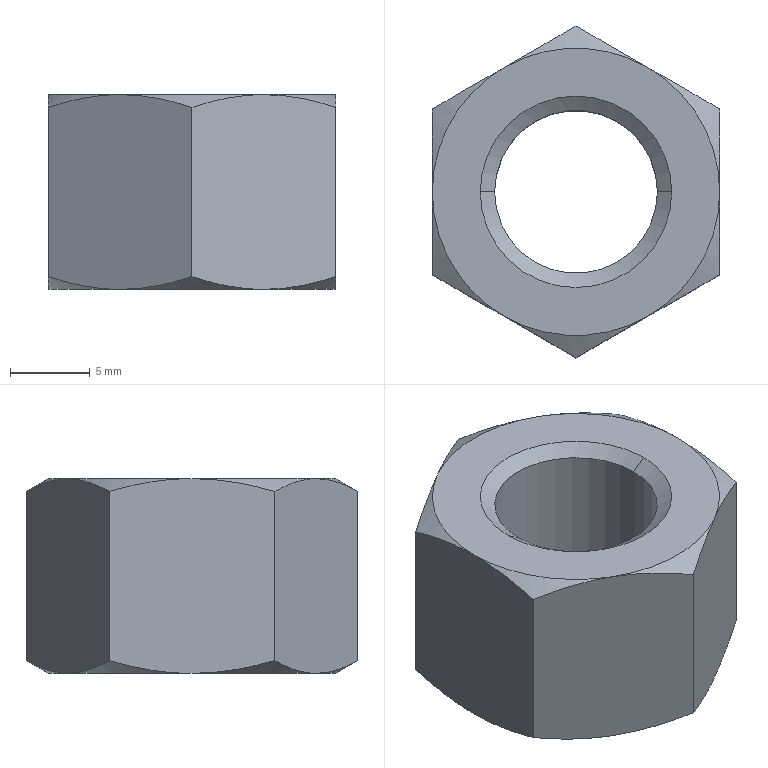Part | STEP file | hex nut gradec_iso_ISO - 4034 - M12 - N | 1 solid | 28 faces | box 18 x 20.785 x 12.2 mm | volume 2394 mm3 | cone 16 | plane 8 | cylinder 4 | commonest cylinder face diameters 10.2 x2 12 x2
STEP:
#1=CARTESIAN_POINT('',(-6.,0.,-12.2));
#2=VERTEX_POINT('',#1);
#3=CARTESIAN_POINT('',(6.,0.,-12.2));
#4=VERTEX_POINT('',#3);
#5=CARTESIAN_POINT('',(0.,0.,-12.2));
#6=DIRECTION('',(0.,0.,1.));
#7=DIRECTION('',(-1.,0.,0.));
#8=AXIS2_PLACEMENT_3D('',#5,#6,#7);
#9=CIRCLE('',#8,6.);
#10=EDGE_CURVE('',#2,#4,#9,.T.);
#11=ORIENTED_EDGE('',*,*,#10,.F.);
#12=CARTESIAN_POINT('',(-6.,0.,-12.175));
#13=VERTEX_POINT('',#12);
#14=CARTESIAN_POINT('',(-6.,0.,-25.038));
#15=DIRECTION('',(0.,0.,1.));
#16=VECTOR('',#15,1000.);
#17=LINE('',#14,#16);
#18=EDGE_CURVE('',#2,#13,#17,.T.);
#19=ORIENTED_EDGE('',*,*,#18,.T.);
#20=CARTESIAN_POINT('',(6.,0.,-12.175));
#21=VERTEX_POINT('',#20);
#22=CARTESIAN_POINT('',(0.,0.,-12.175));
#23=DIRECTION('',(0.,0.,1.));
#24=DIRECTION('',(1.,0.,0.));
#25=AXIS2_PLACEMENT_3D('',#22,#23,#24);
#26=CIRCLE('',#25,6.);
#27=EDGE_CURVE('',#13,#21,#26,.T.);
#28=ORIENTED_EDGE('',*,*,#27,.T.);
#29=CARTESIAN_POINT('',(6.,0.,-25.038));
#30=DIRECTION('',(0.,0.,1.));
#31=VECTOR('',#30,1000.);
#32=LINE('',#29,#31);
#33=EDGE_CURVE('',#4,#21,#32,.T.);
#34=ORIENTED_EDGE('',*,*,#33,.F.);
#35=EDGE_LOOP('',(#11,#19,#28,#34));
#36=FACE_OUTER_BOUND('',#35,.T.);
#37=CARTESIAN_POINT('',(0.,0.,-25.038));
#38=DIRECTION('',(0.,0.,1.));
#39=DIRECTION('',(1.,0.,0.));
#40=AXIS2_PLACEMENT_3D('',#37,#38,#39);
#41=CYLINDRICAL_SURFACE('',#40,6.);
#42=ADVANCED_FACE('',(#36),#41,.F.);
#43=CARTESIAN_POINT('',(-5.1,0.,-11.544));
#44=VERTEX_POINT('',#43);
#45=CARTESIAN_POINT('',(5.1,0.,-11.544));
#46=VERTEX_POINT('',#45);
#47=CARTESIAN_POINT('',(0.,0.,-11.544));
#48=DIRECTION('',(0.,0.,1.));
#49=DIRECTION('',(-1.,0.,0.));
#50=AXIS2_PLACEMENT_3D('',#47,#48,#49);
#51=CIRCLE('',#50,5.1);
#52=EDGE_CURVE('',#44,#46,#51,.T.);
#53=ORIENTED_EDGE('',*,*,#52,.T.);
#54=CARTESIAN_POINT('',(6.,0.,-12.175));
#55=DIRECTION('',(0.8192,0.,-0.5736));
#56=VECTOR('',#55,1000.);
#57=LINE('',#54,#56);
#58=EDGE_CURVE('',#46,#21,#57,.T.);
#59=ORIENTED_EDGE('',*,*,#58,.T.);
#60=ORIENTED_EDGE('',*,*,#27,.F.);
#61=CARTESIAN_POINT('',(-6.,0.,-12.175));
#62=DIRECTION('',(-0.8192,0.,-0.5736));
#63=VECTOR('',#62,1000.);
#64=LINE('',#61,#63);
#65=EDGE_CURVE('',#44,#13,#64,.T.);
#66=ORIENTED_EDGE('',*,*,#65,.F.);
#67=EDGE_LOOP('',(#53,#59,#60,#66));
#68=FACE_OUTER_BOUND('',#67,.T.);
#69=CARTESIAN_POINT('',(0.,0.,-12.175));
#70=DIRECTION('',(0.,0.,-1.));
#71=DIRECTION('',(-1.,0.,0.));
#72=AXIS2_PLACEMENT_3D('',#69,#70,#71);
#73=CONICAL_SURFACE('',#72,6.,0.9599);
#74=ADVANCED_FACE('',(#68),#73,.F.);
#75=CARTESIAN_POINT('',(5.1,0.,-0.6302));
#76=VERTEX_POINT('',#75);
#77=CARTESIAN_POINT('',(-5.1,0.,-0.6302));
#78=VERTEX_POINT('',#77);
#79=CARTESIAN_POINT('',(0.,0.,-0.6302));
#80=DIRECTION('',(0.,0.,-1.));
#81=DIRECTION('',(1.,0.,0.));
#82=AXIS2_PLACEMENT_3D('',#79,#80,#81);
#83=CIRCLE('',#82,5.1);
#84=EDGE_CURVE('',#76,#78,#83,.T.);
#85=ORIENTED_EDGE('',*,*,#84,.T.);
#86=CARTESIAN_POINT('',(-6.,0.,0.));
#87=VERTEX_POINT('',#86);
#88=CARTESIAN_POINT('',(-5.01,0.,-0.6932));
#89=DIRECTION('',(-0.8192,0.,0.5736));
#90=VECTOR('',#89,1000.);
#91=LINE('',#88,#90);
#92=EDGE_CURVE('',#78,#87,#91,.T.);
#93=ORIENTED_EDGE('',*,*,#92,.T.);
#94=CARTESIAN_POINT('',(6.,0.,0.));
#95=VERTEX_POINT('',#94);
#96=CARTESIAN_POINT('',(0.,0.,0.));
#97=DIRECTION('',(0.,0.,1.));
#98=DIRECTION('',(1.,0.,0.));
#99=AXIS2_PLACEMENT_3D('',#96,#97,#98);
#100=CIRCLE('',#99,6.);
#101=EDGE_CURVE('',#87,#95,#100,.T.);
#102=ORIENTED_EDGE('',*,*,#101,.T.);
#103=CARTESIAN_POINT('',(5.01,0.,-0.6932));
#104=DIRECTION('',(0.8192,0.,0.5736));
#105=VECTOR('',#104,1000.);
#106=LINE('',#103,#105);
#107=EDGE_CURVE('',#76,#95,#106,.T.);
#108=ORIENTED_EDGE('',*,*,#107,.F.);
#109=EDGE_LOOP('',(#85,#93,#102,#108));
#110=FACE_OUTER_BOUND('',#109,.T.);
#111=CARTESIAN_POINT('',(0.,0.,-0.6932));
#112=DIRECTION('',(0.,0.,1.));
#113=DIRECTION('',(1.,0.,0.));
#114=AXIS2_PLACEMENT_3D('',#111,#112,#113);
#115=CONICAL_SURFACE('',#114,5.01,0.9599);
#116=ADVANCED_FACE('',(#110),#115,.F.);
#117=ORIENTED_EDGE('',*,*,#52,.F.);
#118=CARTESIAN_POINT('',(-5.1,0.,-12.2));
#119=DIRECTION('',(0.,0.,1.));
#120=VECTOR('',#119,1000.);
#121=LINE('',#118,#120);
#122=EDGE_CURVE('',#44,#78,#121,.T.);
#123=ORIENTED_EDGE('',*,*,#122,.T.);
#124=ORIENTED_EDGE('',*,*,#84,.F.);
#125=CARTESIAN_POINT('',(5.1,0.,-12.2));
#126=DIRECTION('',(0.,0.,1.));
#127=VECTOR('',#126,1000.);
#128=LINE('',#125,#127);
#129=EDGE_CURVE('',#46,#76,#128,.T.);
#130=ORIENTED_EDGE('',*,*,#129,.F.);
#131=EDGE_LOOP('',(#117,#123,#124,#130));
#132=FACE_OUTER_BOUND('',#131,.T.);
#133=CARTESIAN_POINT('',(0.,0.,-12.2));
#134=DIRECTION('',(0.,0.,1.));
#135=DIRECTION('',(1.,0.,0.));
#136=AXIS2_PLACEMENT_3D('',#133,#134,#135);
#137=CYLINDRICAL_SURFACE('',#136,5.1);
#138=ADVANCED_FACE('',(#132),#137,.F.);
#139=ORIENTED_EDGE('',*,*,#122,.F.);
#140=CARTESIAN_POINT('',(0.,0.,-11.544));
#141=DIRECTION('',(0.,0.,1.));
#142=DIRECTION('',(-1.,0.,0.));
#143=AXIS2_PLACEMENT_3D('',#140,#141,#142);
#144=CIRCLE('',#143,5.1);
#145=EDGE_CURVE('',#46,#44,#144,.T.);
#146=ORIENTED_EDGE('',*,*,#145,.F.);
#147=ORIENTED_EDGE('',*,*,#129,.T.);
#148=CARTESIAN_POINT('',(0.,0.,-0.6302));
#149=DIRECTION('',(0.,0.,-1.));
#150=DIRECTION('',(1.,0.,0.));
#151=AXIS2_PLACEMENT_3D('',#148,#149,#150);
#152=CIRCLE('',#151,5.1);
#153=EDGE_CURVE('',#78,#76,#152,.T.);
#154=ORIENTED_EDGE('',*,*,#153,.F.);
#155=EDGE_LOOP('',(#139,#146,#147,#154));
#156=FACE_OUTER_BOUND('',#155,.T.);
#157=CARTESIAN_POINT('',(0.,0.,-12.2));
#158=DIRECTION('',(0.,0.,1.));
#159=DIRECTION('',(1.,0.,0.));
#160=AXIS2_PLACEMENT_3D('',#157,#158,#159);
#161=CYLINDRICAL_SURFACE('',#160,5.1);
#162=ADVANCED_FACE('',(#156),#161,.F.);
#163=CARTESIAN_POINT('',(-9.,5.196,-11.396));
#164=VERTEX_POINT('',#163);
#165=CARTESIAN_POINT('',(-9.,5.196,-0.8038));
#166=VERTEX_POINT('',#165);
#167=CARTESIAN_POINT('',(-9.,5.196,-12.2));
#168=DIRECTION('',(0.,0.,1.));
#169=VECTOR('',#168,1000.);
#170=LINE('',#167,#169);
#171=EDGE_CURVE('',#164,#166,#170,.T.);
#172=ORIENTED_EDGE('',*,*,#171,.T.);
#173=CARTESIAN_POINT('',(-4.5,7.794,0.));
#174=VERTEX_POINT('',#173);
#175=CARTESIAN_POINT('',(-9.,5.196,-0.8038));
#176=CARTESIAN_POINT('',(-8.264,5.621,-0.5585));
#177=CARTESIAN_POINT('',(-7.522,6.049,-0.3563));
#178=CARTESIAN_POINT('',(-6.024,6.914,-0.07661));
#179=CARTESIAN_POINT('',(-5.267,7.352,0.));
#180=CARTESIAN_POINT('',(-4.5,7.794,0.));
#181=B_SPLINE_CURVE_WITH_KNOTS('',3,(#175,#176,#177,#178,#179,#180),.UNSPECIFIED.,.F.,.F.,(4,2,4),(0.000000238,0.002629,0.005258),.UNSPECIFIED.);
#182=EDGE_CURVE('',#166,#174,#181,.T.);
#183=ORIENTED_EDGE('',*,*,#182,.T.);
#184=CARTESIAN_POINT('',(0.,10.392,-0.8038));
#185=VERTEX_POINT('',#184);
#186=CARTESIAN_POINT('',(-4.5,7.794,0.));
#187=CARTESIAN_POINT('',(-4.118,8.015,0.));
#188=CARTESIAN_POINT('',(-3.734,8.236,-0.019));
#189=CARTESIAN_POINT('',(-2.976,8.674,-0.09253));
#190=CARTESIAN_POINT('',(-2.599,8.892,-0.147));
#191=CARTESIAN_POINT('',(-1.475,9.541,-0.357));
#192=CARTESIAN_POINT('',(-0.7343,9.968,-0.5591));
#193=CARTESIAN_POINT('',(0.,10.392,-0.8038));
#194=B_SPLINE_CURVE_WITH_KNOTS('',3,(#186,#187,#188,#189,#190,#191,#192,#193),.UNSPECIFIED.,.F.,.F.,(4,2,2,4),(0.005258,0.006567,0.007877,0.0105),.UNSPECIFIED.);
#195=EDGE_CURVE('',#174,#185,#194,.T.);
#196=ORIENTED_EDGE('',*,*,#195,.T.);
#197=CARTESIAN_POINT('',(0.,10.392,-11.396));
#198=VERTEX_POINT('',#197);
#199=CARTESIAN_POINT('',(0.,10.392,-12.2));
#200=DIRECTION('',(0.,0.,1.));
#201=VECTOR('',#200,1000.);
#202=LINE('',#199,#201);
#203=EDGE_CURVE('',#198,#185,#202,.T.);
#204=ORIENTED_EDGE('',*,*,#203,.F.);
#205=CARTESIAN_POINT('',(-4.5,7.794,-12.2));
#206=VERTEX_POINT('',#205);
#207=CARTESIAN_POINT('',(-4.5,7.794,-12.2));
#208=CARTESIAN_POINT('',(-4.118,8.015,-12.2));
#209=CARTESIAN_POINT('',(-3.734,8.236,-12.181));
#210=CARTESIAN_POINT('',(-2.976,8.674,-12.107));
#211=CARTESIAN_POINT('',(-2.599,8.892,-12.053));
#212=CARTESIAN_POINT('',(-1.475,9.541,-11.843));
#213=CARTESIAN_POINT('',(-0.7343,9.968,-11.641));
#214=CARTESIAN_POINT('',(0.,10.392,-11.396));
#215=B_SPLINE_CURVE_WITH_KNOTS('',3,(#207,#208,#209,#210,#211,#212,#213,#214),.UNSPECIFIED.,.F.,.F.,(4,2,2,4),(0.005258,0.006567,0.007877,0.0105),.UNSPECIFIED.);
#216=EDGE_CURVE('',#206,#198,#215,.T.);
#217=ORIENTED_EDGE('',*,*,#216,.F.);
#218=CARTESIAN_POINT('',(-9.,5.196,-11.396));
#219=CARTESIAN_POINT('',(-8.264,5.621,-11.642));
#220=CARTESIAN_POINT('',(-7.522,6.049,-11.844));
#221=CARTESIAN_POINT('',(-6.024,6.914,-12.123));
#222=CARTESIAN_POINT('',(-5.267,7.352,-12.2));
#223=CARTESIAN_POINT('',(-4.5,7.794,-12.2));
#224=B_SPLINE_CURVE_WITH_KNOTS('',3,(#218,#219,#220,#221,#222,#223),.UNSPECIFIED.,.F.,.F.,(4,2,4),(0.000000238,0.002629,0.005258),.UNSPECIFIED.);
#225=EDGE_CURVE('',#164,#206,#224,.T.);
#226=ORIENTED_EDGE('',*,*,#225,.F.);
#227=EDGE_LOOP('',(#172,#183,#196,#204,#217,#226));
#228=FACE_OUTER_BOUND('',#227,.T.);
#229=CARTESIAN_POINT('',(0.,10.392,-12.2));
#230=DIRECTION('',(-0.5,0.866,0.));
#231=DIRECTION('',(-0.866,-0.5,0.));
#232=AXIS2_PLACEMENT_3D('',#229,#230,#231);
#233=PLANE('',#232);
#234=ADVANCED_FACE('',(#228),#233,.T.);
#235=ORIENTED_EDGE('',*,*,#203,.T.);
#236=CARTESIAN_POINT('',(4.5,7.794,0.));
#237=VERTEX_POINT('',#236);
#238=CARTESIAN_POINT('',(0.,10.392,-0.8038));
#239=CARTESIAN_POINT('',(0.7361,9.967,-0.5585));
#240=CARTESIAN_POINT('',(1.478,9.539,-0.3563));
#241=CARTESIAN_POINT('',(2.976,8.674,-0.07661));
#242=CARTESIAN_POINT('',(3.733,8.237,0.));
#243=CARTESIAN_POINT('',(4.5,7.794,0.));
#244=B_SPLINE_CURVE_WITH_KNOTS('',3,(#238,#239,#240,#241,#242,#243),.UNSPECIFIED.,.F.,.F.,(4,2,4),(0.000000238,0.002629,0.005258),.UNSPECIFIED.);
#245=EDGE_CURVE('',#185,#237,#244,.T.);
#246=ORIENTED_EDGE('',*,*,#245,.T.);
#247=CARTESIAN_POINT('',(9.,5.196,-0.8038));
#248=VERTEX_POINT('',#247);
#249=CARTESIAN_POINT('',(4.5,7.794,0.));
#250=CARTESIAN_POINT('',(4.882,7.574,0.));
#251=CARTESIAN_POINT('',(5.266,7.352,-0.019));
#252=CARTESIAN_POINT('',(6.024,6.914,-0.09253));
#253=CARTESIAN_POINT('',(6.401,6.697,-0.147));
#254=CARTESIAN_POINT('',(7.525,6.048,-0.357));
#255=CARTESIAN_POINT('',(8.266,5.62,-0.5591));
#256=CARTESIAN_POINT('',(9.,5.196,-0.8038));
#257=B_SPLINE_CURVE_WITH_KNOTS('',3,(#249,#250,#251,#252,#253,#254,#255,#256),.UNSPECIFIED.,.F.,.F.,(4,2,2,4),(0.005258,0.006567,0.007877,0.0105),.UNSPECIFIED.);
#258=EDGE_CURVE('',#237,#248,#257,.T.);
#259=ORIENTED_EDGE('',*,*,#258,.T.);
#260=CARTESIAN_POINT('',(9.,5.196,-11.396));
#261=VERTEX_POINT('',#260);
#262=CARTESIAN_POINT('',(9.,5.196,-12.2));
#263=DIRECTION('',(0.,0.,1.));
#264=VECTOR('',#263,1000.);
#265=LINE('',#262,#264);
#266=EDGE_CURVE('',#261,#248,#265,.T.);
#267=ORIENTED_EDGE('',*,*,#266,.F.);
#268=CARTESIAN_POINT('',(4.5,7.794,-12.2));
#269=VERTEX_POINT('',#268);
#270=CARTESIAN_POINT('',(4.5,7.794,-12.2));
#271=CARTESIAN_POINT('',(4.882,7.574,-12.2));
#272=CARTESIAN_POINT('',(5.266,7.352,-12.181));
#273=CARTESIAN_POINT('',(6.024,6.914,-12.107));
#274=CARTESIAN_POINT('',(6.401,6.697,-12.053));
#275=CARTESIAN_POINT('',(7.525,6.048,-11.843));
#276=CARTESIAN_POINT('',(8.266,5.62,-11.641));
#277=CARTESIAN_POINT('',(9.,5.196,-11.396));
#278=B_SPLINE_CURVE_WITH_KNOTS('',3,(#270,#271,#272,#273,#274,#275,#276,#277),.UNSPECIFIED.,.F.,.F.,(4,2,2,4),(0.005258,0.006567,0.007877,0.0105),.UNSPECIFIED.);
#279=EDGE_CURVE('',#269,#261,#278,.T.);
#280=ORIENTED_EDGE('',*,*,#279,.F.);
#281=CARTESIAN_POINT('',(0.,10.392,-11.396));
#282=CARTESIAN_POINT('',(0.7361,9.967,-11.642));
#283=CARTESIAN_POINT('',(1.478,9.539,-11.844));
#284=CARTESIAN_POINT('',(2.976,8.674,-12.123));
#285=CARTESIAN_POINT('',(3.733,8.237,-12.2));
#286=CARTESIAN_POINT('',(4.5,7.794,-12.2));
#287=B_SPLINE_CURVE_WITH_KNOTS('',3,(#281,#282,#283,#284,#285,#286),.UNSPECIFIED.,.F.,.F.,(4,2,4),(0.000000238,0.002629,0.005258),.UNSPECIFIED.);
#288=EDGE_CURVE('',#198,#269,#287,.T.);
#289=ORIENTED_EDGE('',*,*,#288,.F.);
#290=EDGE_LOOP('',(#235,#246,#259,#267,#280,#289));
#291=FACE_OUTER_BOUND('',#290,.T.);
#292=CARTESIAN_POINT('',(9.,5.196,-12.2));
#293=DIRECTION('',(0.5,0.866,0.));
#294=DIRECTION('',(-0.866,0.5,0.));
#295=AXIS2_PLACEMENT_3D('',#292,#293,#294);
#296=PLANE('',#295);
#297=ADVANCED_FACE('',(#291),#296,.T.);
#298=CARTESIAN_POINT('',(9.,-5.196,-0.8038));
#299=VERTEX_POINT('',#298);
#300=CARTESIAN_POINT('',(9.,0.,0.));
#301=VERTEX_POINT('',#300);
#302=CARTESIAN_POINT('',(9.,-5.196,-0.8038));
#303=CARTESIAN_POINT('',(9.,-4.351,-0.5599));
#304=CARTESIAN_POINT('',(9.,-3.485,-0.3553));
#305=CARTESIAN_POINT('',(9.,-1.75,-0.07547));
#306=CARTESIAN_POINT('',(9.,-0.8781,0.));
#307=CARTESIAN_POINT('',(9.,0.,0.));
#308=B_SPLINE_CURVE_WITH_KNOTS('',3,(#302,#303,#304,#305,#306,#307),.UNSPECIFIED.,.F.,.F.,(4,2,4),(0.009271,0.0119,0.01453),.UNSPECIFIED.);
#309=EDGE_CURVE('',#299,#301,#308,.T.);
#310=ORIENTED_EDGE('',*,*,#309,.F.);
#311=CARTESIAN_POINT('',(9.,-5.196,-11.396));
#312=VERTEX_POINT('',#311);
#313=CARTESIAN_POINT('',(9.,-5.196,-12.2));
#314=DIRECTION('',(0.,0.,1.));
#315=VECTOR('',#314,1000.);
#316=LINE('',#313,#315);
#317=EDGE_CURVE('',#312,#299,#316,.T.);
#318=ORIENTED_EDGE('',*,*,#317,.F.);
#319=CARTESIAN_POINT('',(9.,0.,-12.2));
#320=VERTEX_POINT('',#319);
#321=CARTESIAN_POINT('',(9.,-5.196,-11.396));
#322=CARTESIAN_POINT('',(9.,-4.351,-11.64));
#323=CARTESIAN_POINT('',(9.,-3.485,-11.845));
#324=CARTESIAN_POINT('',(9.,-1.75,-12.125));
#325=CARTESIAN_POINT('',(9.,-0.8781,-12.2));
#326=CARTESIAN_POINT('',(9.,0.,-12.2));
#327=B_SPLINE_CURVE_WITH_KNOTS('',3,(#321,#322,#323,#324,#325,#326),.UNSPECIFIED.,.F.,.F.,(4,2,4),(0.009271,0.0119,0.01453),.UNSPECIFIED.);
#328=EDGE_CURVE('',#312,#320,#327,.T.);
#329=ORIENTED_EDGE('',*,*,#328,.T.);
#330=CARTESIAN_POINT('',(9.,0.,-12.2));
#331=CARTESIAN_POINT('',(9.,0.8786,-12.2));
#332=CARTESIAN_POINT('',(9.,1.769,-12.122));
#333=CARTESIAN_POINT('',(9.,3.505,-11.841));
#334=CARTESIAN_POINT('',(9.,4.356,-11.639));
#335=CARTESIAN_POINT('',(9.,5.196,-11.396));
#336=B_SPLINE_CURVE_WITH_KNOTS('',3,(#330,#331,#332,#333,#334,#335),.UNSPECIFIED.,.F.,.F.,(4,2,4),(0.01453,0.01716,0.01979),.UNSPECIFIED.);
#337=EDGE_CURVE('',#320,#261,#336,.T.);
#338=ORIENTED_EDGE('',*,*,#337,.T.);
#339=ORIENTED_EDGE('',*,*,#266,.T.);
#340=CARTESIAN_POINT('',(9.,0.,0.));
#341=CARTESIAN_POINT('',(9.,0.8786,0.));
#342=CARTESIAN_POINT('',(9.,1.769,-0.07756));
#343=CARTESIAN_POINT('',(9.,3.505,-0.3593));
#344=CARTESIAN_POINT('',(9.,4.356,-0.5613));
#345=CARTESIAN_POINT('',(9.,5.196,-0.8038));
#346=B_SPLINE_CURVE_WITH_KNOTS('',3,(#340,#341,#342,#343,#344,#345),.UNSPECIFIED.,.F.,.F.,(4,2,4),(0.01453,0.01716,0.01979),.UNSPECIFIED.);
#347=EDGE_CURVE('',#301,#248,#346,.T.);
#348=ORIENTED_EDGE('',*,*,#347,.F.);
#349=EDGE_LOOP('',(#310,#318,#329,#338,#339,#348));
#350=FACE_OUTER_BOUND('',#349,.T.);
#351=CARTESIAN_POINT('',(9.,5.196,-12.2));
#352=DIRECTION('',(-1.,0.,0.));
#353=DIRECTION('',(0.,0.,1.));
#354=AXIS2_PLACEMENT_3D('',#351,#352,#353);
#355=PLANE('',#354);
#356=ADVANCED_FACE('',(#350),#355,.F.);
#357=ORIENTED_EDGE('',*,*,#317,.T.);
#358=CARTESIAN_POINT('',(4.5,-7.794,0.));
#359=VERTEX_POINT('',#358);
#360=CARTESIAN_POINT('',(9.,-5.196,-0.8038));
#361=CARTESIAN_POINT('',(8.264,-5.621,-0.5585));
#362=CARTESIAN_POINT('',(7.522,-6.049,-0.3563));
#363=CARTESIAN_POINT('',(6.024,-6.914,-0.07661));
#364=CARTESIAN_POINT('',(5.267,-7.352,0.));
#365=CARTESIAN_POINT('',(4.5,-7.794,0.));
#366=B_SPLINE_CURVE_WITH_KNOTS('',3,(#360,#361,#362,#363,#364,#365),.UNSPECIFIED.,.F.,.F.,(4,2,4),(0.000000238,0.002629,0.005258),.UNSPECIFIED.);
#367=EDGE_CURVE('',#299,#359,#366,.T.);
#368=ORIENTED_EDGE('',*,*,#367,.T.);
#369=CARTESIAN_POINT('',(0.,-10.392,-0.8038));
#370=VERTEX_POINT('',#369);
#371=CARTESIAN_POINT('',(4.5,-7.794,0.));
#372=CARTESIAN_POINT('',(4.118,-8.015,0.));
#373=CARTESIAN_POINT('',(3.734,-8.236,-0.019));
#374=CARTESIAN_POINT('',(2.976,-8.674,-0.09253));
#375=CARTESIAN_POINT('',(2.599,-8.892,-0.147));
#376=CARTESIAN_POINT('',(1.475,-9.541,-0.357));
#377=CARTESIAN_POINT('',(0.7343,-9.968,-0.5591));
#378=CARTESIAN_POINT('',(0.,-10.392,-0.8038));
#379=B_SPLINE_CURVE_WITH_KNOTS('',3,(#371,#372,#373,#374,#375,#376,#377,#378),.UNSPECIFIED.,.F.,.F.,(4,2,2,4),(0.005258,0.006567,0.007877,0.0105),.UNSPECIFIED.);
#380=EDGE_CURVE('',#359,#370,#379,.T.);
#381=ORIENTED_EDGE('',*,*,#380,.T.);
#382=CARTESIAN_POINT('',(0.,-10.392,-11.396));
#383=VERTEX_POINT('',#382);
#384=CARTESIAN_POINT('',(0.,-10.392,-12.2));
#385=DIRECTION('',(0.,0.,1.));
#386=VECTOR('',#385,1000.);
#387=LINE('',#384,#386);
#388=EDGE_CURVE('',#383,#370,#387,.T.);
#389=ORIENTED_EDGE('',*,*,#388,.F.);
#390=CARTESIAN_POINT('',(4.5,-7.794,-12.2));
#391=VERTEX_POINT('',#390);
#392=CARTESIAN_POINT('',(4.5,-7.794,-12.2));
#393=CARTESIAN_POINT('',(4.118,-8.015,-12.2));
#394=CARTESIAN_POINT('',(3.734,-8.236,-12.181));
#395=CARTESIAN_POINT('',(2.976,-8.674,-12.107));
#396=CARTESIAN_POINT('',(2.599,-8.892,-12.053));
#397=CARTESIAN_POINT('',(1.475,-9.541,-11.843));
#398=CARTESIAN_POINT('',(0.7343,-9.968,-11.641));
#399=CARTESIAN_POINT('',(0.,-10.392,-11.396));
#400=B_SPLINE_CURVE_WITH_KNOTS('',3,(#392,#393,#394,#395,#396,#397,#398,#399),.UNSPECIFIED.,.F.,.F.,(4,2,2,4),(0.005258,0.006567,0.007877,0.0105),.UNSPECIFIED.);
#401=EDGE_CURVE('',#391,#383,#400,.T.);
#402=ORIENTED_EDGE('',*,*,#401,.F.);
#403=CARTESIAN_POINT('',(9.,-5.196,-11.396));
#404=CARTESIAN_POINT('',(8.264,-5.621,-11.642));
#405=CARTESIAN_POINT('',(7.522,-6.049,-11.844));
#406=CARTESIAN_POINT('',(6.024,-6.914,-12.123));
#407=CARTESIAN_POINT('',(5.267,-7.352,-12.2));
#408=CARTESIAN_POINT('',(4.5,-7.794,-12.2));
#409=B_SPLINE_CURVE_WITH_KNOTS('',3,(#403,#404,#405,#406,#407,#408),.UNSPECIFIED.,.F.,.F.,(4,2,4),(0.000000238,0.002629,0.005258),.UNSPECIFIED.);
#410=EDGE_CURVE('',#312,#391,#409,.T.);
#411=ORIENTED_EDGE('',*,*,#410,.F.);
#412=EDGE_LOOP('',(#357,#368,#381,#389,#402,#411));
#413=FACE_OUTER_BOUND('',#412,.T.);
#414=CARTESIAN_POINT('',(0.,-10.392,-12.2));
#415=DIRECTION('',(0.5,-0.866,0.));
#416=DIRECTION('',(0.866,0.5,0.));
#417=AXIS2_PLACEMENT_3D('',#414,#415,#416);
#418=PLANE('',#417);
#419=ADVANCED_FACE('',(#413),#418,.T.);
#420=ORIENTED_EDGE('',*,*,#388,.T.);
#421=CARTESIAN_POINT('',(-4.5,-7.794,0.));
#422=VERTEX_POINT('',#421);
#423=CARTESIAN_POINT('',(0.,-10.392,-0.8038));
#424=CARTESIAN_POINT('',(-0.7361,-9.967,-0.5585));
#425=CARTESIAN_POINT('',(-1.478,-9.539,-0.3563));
#426=CARTESIAN_POINT('',(-2.976,-8.674,-0.07661));
#427=CARTESIAN_POINT('',(-3.733,-8.237,0.));
#428=CARTESIAN_POINT('',(-4.5,-7.794,0.));
#429=B_SPLINE_CURVE_WITH_KNOTS('',3,(#423,#424,#425,#426,#427,#428),.UNSPECIFIED.,.F.,.F.,(4,2,4),(0.000000238,0.002629,0.005258),.UNSPECIFIED.);
#430=EDGE_CURVE('',#370,#422,#429,.T.);
#431=ORIENTED_EDGE('',*,*,#430,.T.);
#432=CARTESIAN_POINT('',(-9.,-5.196,-0.8038));
#433=VERTEX_POINT('',#432);
#434=CARTESIAN_POINT('',(-4.5,-7.794,0.));
#435=CARTESIAN_POINT('',(-4.882,-7.574,0.));
#436=CARTESIAN_POINT('',(-5.266,-7.352,-0.019));
#437=CARTESIAN_POINT('',(-6.024,-6.914,-0.09253));
#438=CARTESIAN_POINT('',(-6.401,-6.697,-0.147));
#439=CARTESIAN_POINT('',(-7.525,-6.048,-0.357));
#440=CARTESIAN_POINT('',(-8.266,-5.62,-0.5591));
#441=CARTESIAN_POINT('',(-9.,-5.196,-0.8038));
#442=B_SPLINE_CURVE_WITH_KNOTS('',3,(#434,#435,#436,#437,#438,#439,#440,#441),.UNSPECIFIED.,.F.,.F.,(4,2,2,4),(0.005258,0.006567,0.007877,0.0105),.UNSPECIFIED.);
#443=EDGE_CURVE('',#422,#433,#442,.T.);
#444=ORIENTED_EDGE('',*,*,#443,.T.);
#445=CARTESIAN_POINT('',(-9.,-5.196,-11.396));
#446=VERTEX_POINT('',#445);
#447=CARTESIAN_POINT('',(-9.,-5.196,-12.2));
#448=DIRECTION('',(0.,0.,1.));
#449=VECTOR('',#448,1000.);
#450=LINE('',#447,#449);
#451=EDGE_CURVE('',#446,#433,#450,.T.);
#452=ORIENTED_EDGE('',*,*,#451,.F.);
#453=CARTESIAN_POINT('',(-4.5,-7.794,-12.2));
#454=VERTEX_POINT('',#453);
#455=CARTESIAN_POINT('',(-4.5,-7.794,-12.2));
#456=CARTESIAN_POINT('',(-4.882,-7.574,-12.2));
#457=CARTESIAN_POINT('',(-5.266,-7.352,-12.181));
#458=CARTESIAN_POINT('',(-6.024,-6.914,-12.107));
#459=CARTESIAN_POINT('',(-6.401,-6.697,-12.053));
#460=CARTESIAN_POINT('',(-7.525,-6.048,-11.843));
#461=CARTESIAN_POINT('',(-8.266,-5.62,-11.641));
#462=CARTESIAN_POINT('',(-9.,-5.196,-11.396));
#463=B_SPLINE_CURVE_WITH_KNOTS('',3,(#455,#456,#457,#458,#459,#460,#461,#462),.UNSPECIFIED.,.F.,.F.,(4,2,2,4),(0.005258,0.006567,0.007877,0.0105),.UNSPECIFIED.);
#464=EDGE_CURVE('',#454,#446,#463,.T.);
#465=ORIENTED_EDGE('',*,*,#464,.F.);
#466=CARTESIAN_POINT('',(0.,-10.392,-11.396));
#467=CARTESIAN_POINT('',(-0.7361,-9.967,-11.642));
#468=CARTESIAN_POINT('',(-1.478,-9.539,-11.844));
#469=CARTESIAN_POINT('',(-2.976,-8.674,-12.123));
#470=CARTESIAN_POINT('',(-3.733,-8.237,-12.2));
#471=CARTESIAN_POINT('',(-4.5,-7.794,-12.2));
#472=B_SPLINE_CURVE_WITH_KNOTS('',3,(#466,#467,#468,#469,#470,#471),.UNSPECIFIED.,.F.,.F.,(4,2,4),(0.000000238,0.002629,0.005258),.UNSPECIFIED.);
#473=EDGE_CURVE('',#383,#454,#472,.T.);
#474=ORIENTED_EDGE('',*,*,#473,.F.);
#475=EDGE_LOOP('',(#420,#431,#444,#452,#465,#474));
#476=FACE_OUTER_BOUND('',#475,.T.);
#477=CARTESIAN_POINT('',(-9.,-5.196,-12.2));
#478=DIRECTION('',(-0.5,-0.866,0.));
#479=DIRECTION('',(0.866,-0.5,0.));
#480=AXIS2_PLACEMENT_3D('',#477,#478,#479);
#481=PLANE('',#480);
#482=ADVANCED_FACE('',(#476),#481,.T.);
#483=ORIENTED_EDGE('',*,*,#451,.T.);
#484=CARTESIAN_POINT('',(-9.,0.,0.));
#485=VERTEX_POINT('',#484);
#486=CARTESIAN_POINT('',(-9.,-5.196,-0.8038));
#487=CARTESIAN_POINT('',(-9.,-4.351,-0.5599));
#488=CARTESIAN_POINT('',(-9.,-3.485,-0.3553));
#489=CARTESIAN_POINT('',(-9.,-1.75,-0.07547));
#490=CARTESIAN_POINT('',(-9.,-0.8781,0.));
#491=CARTESIAN_POINT('',(-9.,0.,0.));
#492=B_SPLINE_CURVE_WITH_KNOTS('',3,(#486,#487,#488,#489,#490,#491),.UNSPECIFIED.,.F.,.F.,(4,2,4),(0.009271,0.0119,0.01453),.UNSPECIFIED.);
#493=EDGE_CURVE('',#433,#485,#492,.T.);
#494=ORIENTED_EDGE('',*,*,#493,.T.);
#495=CARTESIAN_POINT('',(-9.,0.,0.));
#496=CARTESIAN_POINT('',(-9.,0.8786,0.));
#497=CARTESIAN_POINT('',(-9.,1.769,-0.07756));
#498=CARTESIAN_POINT('',(-9.,3.505,-0.3593));
#499=CARTESIAN_POINT('',(-9.,4.356,-0.5613));
#500=CARTESIAN_POINT('',(-9.,5.196,-0.8038));
#501=B_SPLINE_CURVE_WITH_KNOTS('',3,(#495,#496,#497,#498,#499,#500),.UNSPECIFIED.,.F.,.F.,(4,2,4),(0.01453,0.01716,0.01979),.UNSPECIFIED.);
#502=EDGE_CURVE('',#485,#166,#501,.T.);
#503=ORIENTED_EDGE('',*,*,#502,.T.);
#504=ORIENTED_EDGE('',*,*,#171,.F.);
#505=CARTESIAN_POINT('',(-9.,0.,-12.2));
#506=VERTEX_POINT('',#505);
#507=CARTESIAN_POINT('',(-9.,0.,-12.2));
#508=CARTESIAN_POINT('',(-9.,0.8786,-12.2));
#509=CARTESIAN_POINT('',(-9.,1.769,-12.122));
#510=CARTESIAN_POINT('',(-9.,3.505,-11.841));
#511=CARTESIAN_POINT('',(-9.,4.356,-11.639));
#512=CARTESIAN_POINT('',(-9.,5.196,-11.396));
#513=B_SPLINE_CURVE_WITH_KNOTS('',3,(#507,#508,#509,#510,#511,#512),.UNSPECIFIED.,.F.,.F.,(4,2,4),(0.01453,0.01716,0.01979),.UNSPECIFIED.);
#514=EDGE_CURVE('',#506,#164,#513,.T.);
#515=ORIENTED_EDGE('',*,*,#514,.F.);
#516=CARTESIAN_POINT('',(-9.,-5.196,-11.396));
#517=CARTESIAN_POINT('',(-9.,-4.351,-11.64));
#518=CARTESIAN_POINT('',(-9.,-3.485,-11.845));
#519=CARTESIAN_POINT('',(-9.,-1.75,-12.125));
#520=CARTESIAN_POINT('',(-9.,-0.8781,-12.2));
#521=CARTESIAN_POINT('',(-9.,0.,-12.2));
#522=B_SPLINE_CURVE_WITH_KNOTS('',3,(#516,#517,#518,#519,#520,#521),.UNSPECIFIED.,.F.,.F.,(4,2,4),(0.009271,0.0119,0.01453),.UNSPECIFIED.);
#523=EDGE_CURVE('',#446,#506,#522,.T.);
#524=ORIENTED_EDGE('',*,*,#523,.F.);
#525=EDGE_LOOP('',(#483,#494,#503,#504,#515,#524));
#526=FACE_OUTER_BOUND('',#525,.T.);
#527=CARTESIAN_POINT('',(-9.,5.196,-12.2));
#528=DIRECTION('',(-1.,0.,0.));
#529=DIRECTION('',(0.,0.,1.));
#530=AXIS2_PLACEMENT_3D('',#527,#528,#529);
#531=PLANE('',#530);
#532=ADVANCED_FACE('',(#526),#531,.T.);
#533=CARTESIAN_POINT('',(0.,0.,0.));
#534=DIRECTION('',(0.,0.,1.));
#535=DIRECTION('',(1.,0.,0.));
#536=AXIS2_PLACEMENT_3D('',#533,#534,#535);
#537=CIRCLE('',#536,6.);
#538=EDGE_CURVE('',#95,#87,#537,.T.);
#539=ORIENTED_EDGE('',*,*,#538,.F.);
#540=ORIENTED_EDGE('',*,*,#101,.F.);
#541=EDGE_LOOP('',(#539,#540));
#542=FACE_BOUND('',#541,.T.);
#543=CARTESIAN_POINT('',(0.,0.,0.));
#544=DIRECTION('',(0.,0.,-1.));
#545=DIRECTION('',(-1.,0.,0.));
#546=AXIS2_PLACEMENT_3D('',#543,#544,#545);
#547=CIRCLE('',#546,9.);
#548=EDGE_CURVE('',#485,#174,#547,.T.);
#549=ORIENTED_EDGE('',*,*,#548,.F.);
#550=CARTESIAN_POINT('',(0.,0.,0.));
#551=DIRECTION('',(0.,0.,-1.));
#552=DIRECTION('',(-1.,0.,0.));
#553=AXIS2_PLACEMENT_3D('',#550,#551,#552);
#554=CIRCLE('',#553,9.);
#555=EDGE_CURVE('',#422,#485,#554,.T.);
#556=ORIENTED_EDGE('',*,*,#555,.F.);
#557=CARTESIAN_POINT('',(0.,0.,0.));
#558=DIRECTION('',(0.,0.,-1.));
#559=DIRECTION('',(-1.,0.,0.));
#560=AXIS2_PLACEMENT_3D('',#557,#558,#559);
#561=CIRCLE('',#560,9.);
#562=EDGE_CURVE('',#359,#422,#561,.T.);
#563=ORIENTED_EDGE('',*,*,#562,.F.);
#564=CARTESIAN_POINT('',(0.,0.,0.));
#565=DIRECTION('',(0.,0.,-1.));
#566=DIRECTION('',(-1.,0.,0.));
#567=AXIS2_PLACEMENT_3D('',#564,#565,#566);
#568=CIRCLE('',#567,9.);
#569=EDGE_CURVE('',#301,#359,#568,.T.);
#570=ORIENTED_EDGE('',*,*,#569,.F.);
#571=CARTESIAN_POINT('',(0.,0.,0.));
#572=DIRECTION('',(0.,0.,1.));
#573=DIRECTION('',(1.,0.,0.));
#574=AXIS2_PLACEMENT_3D('',#571,#572,#573);
#575=CIRCLE('',#574,9.);
#576=EDGE_CURVE('',#301,#237,#575,.T.);
#577=ORIENTED_EDGE('',*,*,#576,.T.);
#578=CARTESIAN_POINT('',(0.,0.,0.));
#579=DIRECTION('',(0.,0.,-1.));
#580=DIRECTION('',(-1.,0.,0.));
#581=AXIS2_PLACEMENT_3D('',#578,#579,#580);
#582=CIRCLE('',#581,9.);
#583=EDGE_CURVE('',#174,#237,#582,.T.);
#584=ORIENTED_EDGE('',*,*,#583,.F.);
#585=EDGE_LOOP('',(#549,#556,#563,#570,#577,#584));
#586=FACE_OUTER_BOUND('',#585,.T.);
#587=CARTESIAN_POINT('',(0.,10.392,0.));
#588=DIRECTION('',(0.,0.,-1.));
#589=DIRECTION('',(-1.,0.,0.));
#590=AXIS2_PLACEMENT_3D('',#587,#588,#589);
#591=PLANE('',#590);
#592=ADVANCED_FACE('',(#542,#586),#591,.F.);
#593=CARTESIAN_POINT('',(0.,0.,-12.2));
#594=DIRECTION('',(0.,0.,1.));
#595=DIRECTION('',(-1.,0.,0.));
#596=AXIS2_PLACEMENT_3D('',#593,#594,#595);
#597=CIRCLE('',#596,6.);
#598=EDGE_CURVE('',#4,#2,#597,.T.);
#599=ORIENTED_EDGE('',*,*,#598,.T.);
#600=ORIENTED_EDGE('',*,*,#10,.T.);
#601=EDGE_LOOP('',(#599,#600));
#602=FACE_BOUND('',#601,.T.);
#603=CARTESIAN_POINT('',(0.,0.,-12.2));
#604=DIRECTION('',(0.,0.,1.));
#605=DIRECTION('',(-1.,0.,0.));
#606=AXIS2_PLACEMENT_3D('',#603,#604,#605);
#607=CIRCLE('',#606,9.);
#608=EDGE_CURVE('',#506,#454,#607,.T.);
#609=ORIENTED_EDGE('',*,*,#608,.F.);
#610=CARTESIAN_POINT('',(0.,0.,-12.2));
#611=DIRECTION('',(0.,0.,1.));
#612=DIRECTION('',(-1.,0.,0.));
#613=AXIS2_PLACEMENT_3D('',#610,#611,#612);
#614=CIRCLE('',#613,9.);
#615=EDGE_CURVE('',#206,#506,#614,.T.);
#616=ORIENTED_EDGE('',*,*,#615,.F.);
#617=CARTESIAN_POINT('',(0.,0.,-12.2));
#618=DIRECTION('',(0.,0.,1.));
#619=DIRECTION('',(-1.,0.,0.));
#620=AXIS2_PLACEMENT_3D('',#617,#618,#619);
#621=CIRCLE('',#620,9.);
#622=EDGE_CURVE('',#269,#206,#621,.T.);
#623=ORIENTED_EDGE('',*,*,#622,.F.);
#624=CARTESIAN_POINT('',(0.,0.,-12.2));
#625=DIRECTION('',(0.,0.,1.));
#626=DIRECTION('',(1.,0.,0.));
#627=AXIS2_PLACEMENT_3D('',#624,#625,#626);
#628=CIRCLE('',#627,9.);
#629=EDGE_CURVE('',#320,#269,#628,.T.);
#630=ORIENTED_EDGE('',*,*,#629,.F.);
#631=CARTESIAN_POINT('',(0.,0.,-12.2));
#632=DIRECTION('',(0.,0.,1.));
#633=DIRECTION('',(-1.,0.,0.));
#634=AXIS2_PLACEMENT_3D('',#631,#632,#633);
#635=CIRCLE('',#634,9.);
#636=EDGE_CURVE('',#391,#320,#635,.T.);
#637=ORIENTED_EDGE('',*,*,#636,.F.);
#638=CARTESIAN_POINT('',(0.,0.,-12.2));
#639=DIRECTION('',(0.,0.,1.));
#640=DIRECTION('',(-1.,0.,0.));
#641=AXIS2_PLACEMENT_3D('',#638,#639,#640);
#642=CIRCLE('',#641,9.);
#643=EDGE_CURVE('',#454,#391,#642,.T.);
#644=ORIENTED_EDGE('',*,*,#643,.F.);
#645=EDGE_LOOP('',(#609,#616,#623,#630,#637,#644));
#646=FACE_OUTER_BOUND('',#645,.T.);
#647=CARTESIAN_POINT('',(0.,10.392,-12.2));
#648=DIRECTION('',(0.,0.,-1.));
#649=DIRECTION('',(-1.,0.,0.));
#650=AXIS2_PLACEMENT_3D('',#647,#648,#649);
#651=PLANE('',#650);
#652=ADVANCED_FACE('',(#602,#646),#651,.T.);
#653=ORIENTED_EDGE('',*,*,#225,.T.);
#654=ORIENTED_EDGE('',*,*,#615,.T.);
#655=ORIENTED_EDGE('',*,*,#514,.T.);
#656=EDGE_LOOP('',(#653,#654,#655));
#657=FACE_OUTER_BOUND('',#656,.T.);
#658=CARTESIAN_POINT('',(0.,0.,-12.2));
#659=DIRECTION('',(0.,0.,1.));
#660=DIRECTION('',(1.,0.,0.));
#661=AXIS2_PLACEMENT_3D('',#658,#659,#660);
#662=CONICAL_SURFACE('',#661,9.,1.047);
#663=ADVANCED_FACE('',(#657),#662,.T.);
#664=ORIENTED_EDGE('',*,*,#216,.T.);
#665=ORIENTED_EDGE('',*,*,#288,.T.);
#666=ORIENTED_EDGE('',*,*,#622,.T.);
#667=EDGE_LOOP('',(#664,#665,#666));
#668=FACE_OUTER_BOUND('',#667,.T.);
#669=CARTESIAN_POINT('',(0.,0.,-12.2));
#670=DIRECTION('',(0.,0.,1.));
#671=DIRECTION('',(1.,0.,0.));
#672=AXIS2_PLACEMENT_3D('',#669,#670,#671);
#673=CONICAL_SURFACE('',#672,9.,1.047);
#674=ADVANCED_FACE('',(#668),#673,.T.);
#675=ORIENTED_EDGE('',*,*,#279,.T.);
#676=ORIENTED_EDGE('',*,*,#337,.F.);
#677=ORIENTED_EDGE('',*,*,#629,.T.);
#678=EDGE_LOOP('',(#675,#676,#677));
#679=FACE_OUTER_BOUND('',#678,.T.);
#680=CARTESIAN_POINT('',(0.,0.,-12.2));
#681=DIRECTION('',(0.,0.,1.));
#682=DIRECTION('',(1.,0.,0.));
#683=AXIS2_PLACEMENT_3D('',#680,#681,#682);
#684=CONICAL_SURFACE('',#683,9.,1.047);
#685=ADVANCED_FACE('',(#679),#684,.T.);
#686=ORIENTED_EDGE('',*,*,#410,.T.);
#687=ORIENTED_EDGE('',*,*,#636,.T.);
#688=ORIENTED_EDGE('',*,*,#328,.F.);
#689=EDGE_LOOP('',(#686,#687,#688));
#690=FACE_OUTER_BOUND('',#689,.T.);
#691=CARTESIAN_POINT('',(0.,0.,-12.2));
#692=DIRECTION('',(0.,0.,1.));
#693=DIRECTION('',(1.,0.,0.));
#694=AXIS2_PLACEMENT_3D('',#691,#692,#693);
#695=CONICAL_SURFACE('',#694,9.,1.047);
#696=ADVANCED_FACE('',(#690),#695,.T.);
#697=ORIENTED_EDGE('',*,*,#401,.T.);
#698=ORIENTED_EDGE('',*,*,#473,.T.);
#699=ORIENTED_EDGE('',*,*,#643,.T.);
#700=EDGE_LOOP('',(#697,#698,#699));
#701=FACE_OUTER_BOUND('',#700,.T.);
#702=CARTESIAN_POINT('',(0.,0.,-12.2));
#703=DIRECTION('',(0.,0.,1.));
#704=DIRECTION('',(1.,0.,0.));
#705=AXIS2_PLACEMENT_3D('',#702,#703,#704);
#706=CONICAL_SURFACE('',#705,9.,1.047);
#707=ADVANCED_FACE('',(#701),#706,.T.);
#708=ORIENTED_EDGE('',*,*,#464,.T.);
#709=ORIENTED_EDGE('',*,*,#523,.T.);
#710=ORIENTED_EDGE('',*,*,#608,.T.);
#711=EDGE_LOOP('',(#708,#709,#710));
#712=FACE_OUTER_BOUND('',#711,.T.);
#713=CARTESIAN_POINT('',(0.,0.,-12.2));
#714=DIRECTION('',(0.,0.,1.));
#715=DIRECTION('',(1.,0.,0.));
#716=AXIS2_PLACEMENT_3D('',#713,#714,#715);
#717=CONICAL_SURFACE('',#716,9.,1.047);
#718=ADVANCED_FACE('',(#712),#717,.T.);
#719=ORIENTED_EDGE('',*,*,#555,.T.);
#720=ORIENTED_EDGE('',*,*,#493,.F.);
#721=ORIENTED_EDGE('',*,*,#443,.F.);
#722=EDGE_LOOP('',(#719,#720,#721));
#723=FACE_OUTER_BOUND('',#722,.T.);
#724=CARTESIAN_POINT('',(0.,0.,0.));
#725=DIRECTION('',(0.,0.,-1.));
#726=DIRECTION('',(-1.,0.,0.));
#727=AXIS2_PLACEMENT_3D('',#724,#725,#726);
#728=CONICAL_SURFACE('',#727,9.,1.047);
#729=ADVANCED_FACE('',(#723),#728,.T.);
#730=ORIENTED_EDGE('',*,*,#562,.T.);
#731=ORIENTED_EDGE('',*,*,#430,.F.);
#732=ORIENTED_EDGE('',*,*,#380,.F.);
#733=EDGE_LOOP('',(#730,#731,#732));
#734=FACE_OUTER_BOUND('',#733,.T.);
#735=CARTESIAN_POINT('',(0.,0.,0.));
#736=DIRECTION('',(0.,0.,-1.));
#737=DIRECTION('',(-1.,0.,0.));
#738=AXIS2_PLACEMENT_3D('',#735,#736,#737);
#739=CONICAL_SURFACE('',#738,9.,1.047);
#740=ADVANCED_FACE('',(#734),#739,.T.);
#741=ORIENTED_EDGE('',*,*,#309,.T.);
#742=ORIENTED_EDGE('',*,*,#569,.T.);
#743=ORIENTED_EDGE('',*,*,#367,.F.);
#744=EDGE_LOOP('',(#741,#742,#743));
#745=FACE_OUTER_BOUND('',#744,.T.);
#746=CARTESIAN_POINT('',(0.,0.,0.));
#747=DIRECTION('',(0.,0.,-1.));
#748=DIRECTION('',(-1.,0.,0.));
#749=AXIS2_PLACEMENT_3D('',#746,#747,#748);
#750=CONICAL_SURFACE('',#749,9.,1.047);
#751=ADVANCED_FACE('',(#745),#750,.T.);
#752=ORIENTED_EDGE('',*,*,#576,.F.);
#753=ORIENTED_EDGE('',*,*,#347,.T.);
#754=ORIENTED_EDGE('',*,*,#258,.F.);
#755=EDGE_LOOP('',(#752,#753,#754));
#756=FACE_OUTER_BOUND('',#755,.T.);
#757=CARTESIAN_POINT('',(0.,0.,0.));
#758=DIRECTION('',(0.,0.,-1.));
#759=DIRECTION('',(-1.,0.,0.));
#760=AXIS2_PLACEMENT_3D('',#757,#758,#759);
#761=CONICAL_SURFACE('',#760,9.,1.047);
#762=ADVANCED_FACE('',(#756),#761,.T.);
#763=ORIENTED_EDGE('',*,*,#583,.T.);
#764=ORIENTED_EDGE('',*,*,#245,.F.);
#765=ORIENTED_EDGE('',*,*,#195,.F.);
#766=EDGE_LOOP('',(#763,#764,#765));
#767=FACE_OUTER_BOUND('',#766,.T.);
#768=CARTESIAN_POINT('',(0.,0.,0.));
#769=DIRECTION('',(0.,0.,-1.));
#770=DIRECTION('',(-1.,0.,0.));
#771=AXIS2_PLACEMENT_3D('',#768,#769,#770);
#772=CONICAL_SURFACE('',#771,9.,1.047);
#773=ADVANCED_FACE('',(#767),#772,.T.);
#774=ORIENTED_EDGE('',*,*,#502,.F.);
#775=ORIENTED_EDGE('',*,*,#548,.T.);
#776=ORIENTED_EDGE('',*,*,#182,.F.);
#777=EDGE_LOOP('',(#774,#775,#776));
#778=FACE_OUTER_BOUND('',#777,.T.);
#779=CARTESIAN_POINT('',(0.,0.,0.));
#780=DIRECTION('',(0.,0.,-1.));
#781=DIRECTION('',(-1.,0.,0.));
#782=AXIS2_PLACEMENT_3D('',#779,#780,#781);
#783=CONICAL_SURFACE('',#782,9.,1.047);
#784=ADVANCED_FACE('',(#778),#783,.T.);
#785=ORIENTED_EDGE('',*,*,#92,.F.);
#786=ORIENTED_EDGE('',*,*,#153,.T.);
#787=ORIENTED_EDGE('',*,*,#107,.T.);
#788=ORIENTED_EDGE('',*,*,#538,.T.);
#789=EDGE_LOOP('',(#785,#786,#787,#788));
#790=FACE_OUTER_BOUND('',#789,.T.);
#791=CARTESIAN_POINT('',(0.,0.,-0.6932));
#792=DIRECTION('',(0.,0.,1.));
#793=DIRECTION('',(1.,0.,0.));
#794=AXIS2_PLACEMENT_3D('',#791,#792,#793);
#795=CONICAL_SURFACE('',#794,5.01,0.9599);
#796=ADVANCED_FACE('',(#790),#795,.F.);
#797=ORIENTED_EDGE('',*,*,#58,.F.);
#798=ORIENTED_EDGE('',*,*,#145,.T.);
#799=ORIENTED_EDGE('',*,*,#65,.T.);
#800=CARTESIAN_POINT('',(0.,0.,-12.175));
#801=DIRECTION('',(0.,0.,1.));
#802=DIRECTION('',(1.,0.,0.));
#803=AXIS2_PLACEMENT_3D('',#800,#801,#802);
#804=CIRCLE('',#803,6.);
#805=EDGE_CURVE('',#21,#13,#804,.T.);
#806=ORIENTED_EDGE('',*,*,#805,.F.);
#807=EDGE_LOOP('',(#797,#798,#799,#806));
#808=FACE_OUTER_BOUND('',#807,.T.);
#809=CARTESIAN_POINT('',(0.,0.,-12.175));
#810=DIRECTION('',(0.,0.,-1.));
#811=DIRECTION('',(-1.,0.,0.));
#812=AXIS2_PLACEMENT_3D('',#809,#810,#811);
#813=CONICAL_SURFACE('',#812,6.,0.9599);
#814=ADVANCED_FACE('',(#808),#813,.F.);
#815=ORIENTED_EDGE('',*,*,#18,.F.);
#816=ORIENTED_EDGE('',*,*,#598,.F.);
#817=ORIENTED_EDGE('',*,*,#33,.T.);
#818=ORIENTED_EDGE('',*,*,#805,.T.);
#819=EDGE_LOOP('',(#815,#816,#817,#818));
#820=FACE_OUTER_BOUND('',#819,.T.);
#821=CARTESIAN_POINT('',(0.,0.,-25.038));
#822=DIRECTION('',(0.,0.,1.));
#823=DIRECTION('',(1.,0.,0.));
#824=AXIS2_PLACEMENT_3D('',#821,#822,#823);
#825=CYLINDRICAL_SURFACE('',#824,6.);
#826=ADVANCED_FACE('',(#820),#825,.F.);
#827=CLOSED_SHELL('',(#42,#74,#116,#138,#162,#234,#297,#356,#419,#482,#532,#592,#652,#663,#674,#685,#696,#707,#718,#729,#740,#751,#762,#773,#784,#796,#814,#826));
#828=MANIFOLD_SOLID_BREP('',#827);
#829=CARTESIAN_POINT('',(0.,0.,0.));
#830=DIRECTION('',(0.,0.,1.));
#831=DIRECTION('',(1.,0.,0.));
#832=AXIS2_PLACEMENT_3D('',#829,#830,#831);
#833=(LENGTH_UNIT()NAMED_UNIT(*)SI_UNIT(.MILLI.,.METRE.));
#834=UNCERTAINTY_MEASURE_WITH_UNIT(LENGTH_MEASURE(0.00001),#833,'','');
#835=(NAMED_UNIT(*)PLANE_ANGLE_UNIT()SI_UNIT($,.RADIAN.));
#836=(NAMED_UNIT(*)SI_UNIT($,.STERADIAN.)SOLID_ANGLE_UNIT());
#837=(GEOMETRIC_REPRESENTATION_CONTEXT(3)GLOBAL_UNCERTAINTY_ASSIGNED_CONTEXT((#834))GLOBAL_UNIT_ASSIGNED_CONTEXT((#833,#835,#836))REPRESENTATION_CONTEXT('',''));
#838=ADVANCED_BREP_SHAPE_REPRESENTATION('',(#828,#832),#837);